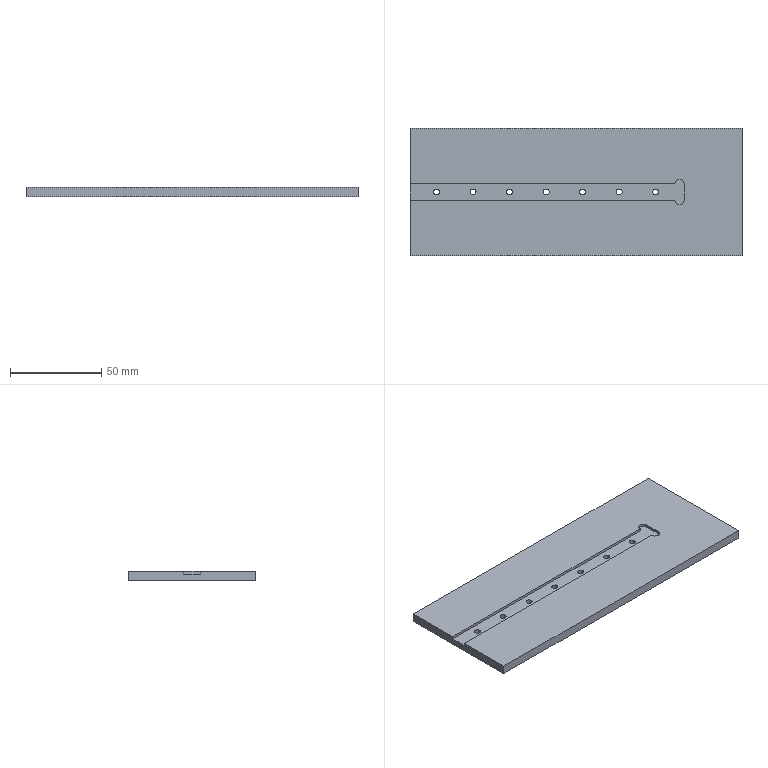Part | STEP file | Handling mechanism support plate | 1 solid | 26 faces | box 181.74 x 70 x 5 mm | volume 61345 mm3 | cylinder 16 | plane 10 | commonest cylinder face diameters 3.3 x14 5 x2
STEP:
#1=CARTESIAN_POINT('',(45.28,0.,0.));
#2=VERTEX_POINT('',#1);
#3=CARTESIAN_POINT('',(41.98,0.,0.));
#4=VERTEX_POINT('',#3);
#5=CARTESIAN_POINT('',(43.63,0.,0.));
#6=DIRECTION('',(0.,0.,-1.));
#7=DIRECTION('',(-1.,0.,0.));
#8=AXIS2_PLACEMENT_3D('',#5,#6,#7);
#9=CIRCLE('',#8,1.65);
#10=EDGE_CURVE('',#2,#4,#9,.T.);
#11=ORIENTED_EDGE('',*,*,#10,.T.);
#12=CARTESIAN_POINT('',(41.98,0.,3.5));
#13=VERTEX_POINT('',#12);
#14=CARTESIAN_POINT('',(41.98,0.,5.));
#15=DIRECTION('',(0.,0.,1.));
#16=VECTOR('',#15,1000.);
#17=LINE('',#14,#16);
#18=EDGE_CURVE('',#4,#13,#17,.T.);
#19=ORIENTED_EDGE('',*,*,#18,.T.);
#20=CARTESIAN_POINT('',(45.28,0.,3.5));
#21=VERTEX_POINT('',#20);
#22=CARTESIAN_POINT('',(43.63,0.,3.5));
#23=DIRECTION('',(0.,0.,1.));
#24=DIRECTION('',(1.,0.,0.));
#25=AXIS2_PLACEMENT_3D('',#22,#23,#24);
#26=CIRCLE('',#25,1.65);
#27=EDGE_CURVE('',#13,#21,#26,.T.);
#28=ORIENTED_EDGE('',*,*,#27,.T.);
#29=CARTESIAN_POINT('',(45.28,0.,5.));
#30=DIRECTION('',(0.,0.,1.));
#31=VECTOR('',#30,1000.);
#32=LINE('',#29,#31);
#33=EDGE_CURVE('',#2,#21,#32,.T.);
#34=ORIENTED_EDGE('',*,*,#33,.F.);
#35=EDGE_LOOP('',(#11,#19,#28,#34));
#36=FACE_OUTER_BOUND('',#35,.T.);
#37=CARTESIAN_POINT('',(43.63,0.,5.));
#38=DIRECTION('',(0.,0.,1.));
#39=DIRECTION('',(1.,0.,0.));
#40=AXIS2_PLACEMENT_3D('',#37,#38,#39);
#41=CYLINDRICAL_SURFACE('',#40,1.65);
#42=ADVANCED_FACE('',(#36),#41,.F.);
#43=CARTESIAN_POINT('',(25.28,0.,0.));
#44=VERTEX_POINT('',#43);
#45=CARTESIAN_POINT('',(21.98,0.,0.));
#46=VERTEX_POINT('',#45);
#47=CARTESIAN_POINT('',(23.63,0.,0.));
#48=DIRECTION('',(0.,0.,-1.));
#49=DIRECTION('',(-1.,0.,0.));
#50=AXIS2_PLACEMENT_3D('',#47,#48,#49);
#51=CIRCLE('',#50,1.65);
#52=EDGE_CURVE('',#44,#46,#51,.T.);
#53=ORIENTED_EDGE('',*,*,#52,.T.);
#54=CARTESIAN_POINT('',(21.98,0.,3.5));
#55=VERTEX_POINT('',#54);
#56=CARTESIAN_POINT('',(21.98,0.,5.));
#57=DIRECTION('',(0.,0.,1.));
#58=VECTOR('',#57,1000.);
#59=LINE('',#56,#58);
#60=EDGE_CURVE('',#46,#55,#59,.T.);
#61=ORIENTED_EDGE('',*,*,#60,.T.);
#62=CARTESIAN_POINT('',(25.28,0.,3.5));
#63=VERTEX_POINT('',#62);
#64=CARTESIAN_POINT('',(23.63,0.,3.5));
#65=DIRECTION('',(0.,0.,1.));
#66=DIRECTION('',(1.,0.,0.));
#67=AXIS2_PLACEMENT_3D('',#64,#65,#66);
#68=CIRCLE('',#67,1.65);
#69=EDGE_CURVE('',#55,#63,#68,.T.);
#70=ORIENTED_EDGE('',*,*,#69,.T.);
#71=CARTESIAN_POINT('',(25.28,0.,5.));
#72=DIRECTION('',(0.,0.,1.));
#73=VECTOR('',#72,1000.);
#74=LINE('',#71,#73);
#75=EDGE_CURVE('',#44,#63,#74,.T.);
#76=ORIENTED_EDGE('',*,*,#75,.F.);
#77=EDGE_LOOP('',(#53,#61,#70,#76));
#78=FACE_OUTER_BOUND('',#77,.T.);
#79=CARTESIAN_POINT('',(23.63,0.,5.));
#80=DIRECTION('',(0.,0.,1.));
#81=DIRECTION('',(1.,0.,0.));
#82=AXIS2_PLACEMENT_3D('',#79,#80,#81);
#83=CYLINDRICAL_SURFACE('',#82,1.65);
#84=ADVANCED_FACE('',(#78),#83,.F.);
#85=CARTESIAN_POINT('',(5.28,0.,0.));
#86=VERTEX_POINT('',#85);
#87=CARTESIAN_POINT('',(1.98,0.,0.));
#88=VERTEX_POINT('',#87);
#89=CARTESIAN_POINT('',(3.63,0.,0.));
#90=DIRECTION('',(0.,0.,-1.));
#91=DIRECTION('',(-1.,0.,0.));
#92=AXIS2_PLACEMENT_3D('',#89,#90,#91);
#93=CIRCLE('',#92,1.65);
#94=EDGE_CURVE('',#86,#88,#93,.T.);
#95=ORIENTED_EDGE('',*,*,#94,.T.);
#96=CARTESIAN_POINT('',(1.98,0.,3.5));
#97=VERTEX_POINT('',#96);
#98=CARTESIAN_POINT('',(1.98,0.,5.));
#99=DIRECTION('',(0.,0.,1.));
#100=VECTOR('',#99,1000.);
#101=LINE('',#98,#100);
#102=EDGE_CURVE('',#88,#97,#101,.T.);
#103=ORIENTED_EDGE('',*,*,#102,.T.);
#104=CARTESIAN_POINT('',(5.28,0.,3.5));
#105=VERTEX_POINT('',#104);
#106=CARTESIAN_POINT('',(3.63,0.,3.5));
#107=DIRECTION('',(0.,0.,1.));
#108=DIRECTION('',(1.,0.,0.));
#109=AXIS2_PLACEMENT_3D('',#106,#107,#108);
#110=CIRCLE('',#109,1.65);
#111=EDGE_CURVE('',#97,#105,#110,.T.);
#112=ORIENTED_EDGE('',*,*,#111,.T.);
#113=CARTESIAN_POINT('',(5.28,0.,5.));
#114=DIRECTION('',(0.,0.,1.));
#115=VECTOR('',#114,1000.);
#116=LINE('',#113,#115);
#117=EDGE_CURVE('',#86,#105,#116,.T.);
#118=ORIENTED_EDGE('',*,*,#117,.F.);
#119=EDGE_LOOP('',(#95,#103,#112,#118));
#120=FACE_OUTER_BOUND('',#119,.T.);
#121=CARTESIAN_POINT('',(3.63,0.,5.));
#122=DIRECTION('',(0.,0.,1.));
#123=DIRECTION('',(1.,0.,0.));
#124=AXIS2_PLACEMENT_3D('',#121,#122,#123);
#125=CYLINDRICAL_SURFACE('',#124,1.65);
#126=ADVANCED_FACE('',(#120),#125,.F.);
#127=CARTESIAN_POINT('',(-14.72,0.,0.));
#128=VERTEX_POINT('',#127);
#129=CARTESIAN_POINT('',(-18.02,0.,0.));
#130=VERTEX_POINT('',#129);
#131=CARTESIAN_POINT('',(-16.37,0.,0.));
#132=DIRECTION('',(0.,0.,-1.));
#133=DIRECTION('',(-1.,0.,0.));
#134=AXIS2_PLACEMENT_3D('',#131,#132,#133);
#135=CIRCLE('',#134,1.65);
#136=EDGE_CURVE('',#128,#130,#135,.T.);
#137=ORIENTED_EDGE('',*,*,#136,.T.);
#138=CARTESIAN_POINT('',(-18.02,0.,3.5));
#139=VERTEX_POINT('',#138);
#140=CARTESIAN_POINT('',(-18.02,0.,5.));
#141=DIRECTION('',(0.,0.,1.));
#142=VECTOR('',#141,1000.);
#143=LINE('',#140,#142);
#144=EDGE_CURVE('',#130,#139,#143,.T.);
#145=ORIENTED_EDGE('',*,*,#144,.T.);
#146=CARTESIAN_POINT('',(-14.72,0.,3.5));
#147=VERTEX_POINT('',#146);
#148=CARTESIAN_POINT('',(-16.37,0.,3.5));
#149=DIRECTION('',(0.,0.,1.));
#150=DIRECTION('',(1.,0.,0.));
#151=AXIS2_PLACEMENT_3D('',#148,#149,#150);
#152=CIRCLE('',#151,1.65);
#153=EDGE_CURVE('',#139,#147,#152,.T.);
#154=ORIENTED_EDGE('',*,*,#153,.T.);
#155=CARTESIAN_POINT('',(-14.72,0.,5.));
#156=DIRECTION('',(0.,0.,1.));
#157=VECTOR('',#156,1000.);
#158=LINE('',#155,#157);
#159=EDGE_CURVE('',#128,#147,#158,.T.);
#160=ORIENTED_EDGE('',*,*,#159,.F.);
#161=EDGE_LOOP('',(#137,#145,#154,#160));
#162=FACE_OUTER_BOUND('',#161,.T.);
#163=CARTESIAN_POINT('',(-16.37,0.,5.));
#164=DIRECTION('',(0.,0.,1.));
#165=DIRECTION('',(1.,0.,0.));
#166=AXIS2_PLACEMENT_3D('',#163,#164,#165);
#167=CYLINDRICAL_SURFACE('',#166,1.65);
#168=ADVANCED_FACE('',(#162),#167,.F.);
#169=CARTESIAN_POINT('',(-34.72,0.,0.));
#170=VERTEX_POINT('',#169);
#171=CARTESIAN_POINT('',(-38.02,0.,0.));
#172=VERTEX_POINT('',#171);
#173=CARTESIAN_POINT('',(-36.37,0.,0.));
#174=DIRECTION('',(0.,0.,-1.));
#175=DIRECTION('',(-1.,0.,0.));
#176=AXIS2_PLACEMENT_3D('',#173,#174,#175);
#177=CIRCLE('',#176,1.65);
#178=EDGE_CURVE('',#170,#172,#177,.T.);
#179=ORIENTED_EDGE('',*,*,#178,.T.);
#180=CARTESIAN_POINT('',(-38.02,0.,3.5));
#181=VERTEX_POINT('',#180);
#182=CARTESIAN_POINT('',(-38.02,0.,5.));
#183=DIRECTION('',(0.,0.,1.));
#184=VECTOR('',#183,1000.);
#185=LINE('',#182,#184);
#186=EDGE_CURVE('',#172,#181,#185,.T.);
#187=ORIENTED_EDGE('',*,*,#186,.T.);
#188=CARTESIAN_POINT('',(-34.72,0.,3.5));
#189=VERTEX_POINT('',#188);
#190=CARTESIAN_POINT('',(-36.37,0.,3.5));
#191=DIRECTION('',(0.,0.,1.));
#192=DIRECTION('',(1.,0.,0.));
#193=AXIS2_PLACEMENT_3D('',#190,#191,#192);
#194=CIRCLE('',#193,1.65);
#195=EDGE_CURVE('',#181,#189,#194,.T.);
#196=ORIENTED_EDGE('',*,*,#195,.T.);
#197=CARTESIAN_POINT('',(-34.72,0.,5.));
#198=DIRECTION('',(0.,0.,1.));
#199=VECTOR('',#198,1000.);
#200=LINE('',#197,#199);
#201=EDGE_CURVE('',#170,#189,#200,.T.);
#202=ORIENTED_EDGE('',*,*,#201,.F.);
#203=EDGE_LOOP('',(#179,#187,#196,#202));
#204=FACE_OUTER_BOUND('',#203,.T.);
#205=CARTESIAN_POINT('',(-36.37,0.,5.));
#206=DIRECTION('',(0.,0.,1.));
#207=DIRECTION('',(1.,0.,0.));
#208=AXIS2_PLACEMENT_3D('',#205,#206,#207);
#209=CYLINDRICAL_SURFACE('',#208,1.65);
#210=ADVANCED_FACE('',(#204),#209,.F.);
#211=CARTESIAN_POINT('',(-54.72,0.,0.));
#212=VERTEX_POINT('',#211);
#213=CARTESIAN_POINT('',(-58.02,0.,0.));
#214=VERTEX_POINT('',#213);
#215=CARTESIAN_POINT('',(-56.37,0.,0.));
#216=DIRECTION('',(0.,0.,-1.));
#217=DIRECTION('',(-1.,0.,0.));
#218=AXIS2_PLACEMENT_3D('',#215,#216,#217);
#219=CIRCLE('',#218,1.65);
#220=EDGE_CURVE('',#212,#214,#219,.T.);
#221=ORIENTED_EDGE('',*,*,#220,.T.);
#222=CARTESIAN_POINT('',(-58.02,0.,3.5));
#223=VERTEX_POINT('',#222);
#224=CARTESIAN_POINT('',(-58.02,0.,5.));
#225=DIRECTION('',(0.,0.,1.));
#226=VECTOR('',#225,1000.);
#227=LINE('',#224,#226);
#228=EDGE_CURVE('',#214,#223,#227,.T.);
#229=ORIENTED_EDGE('',*,*,#228,.T.);
#230=CARTESIAN_POINT('',(-54.72,0.,3.5));
#231=VERTEX_POINT('',#230);
#232=CARTESIAN_POINT('',(-56.37,0.,3.5));
#233=DIRECTION('',(0.,0.,1.));
#234=DIRECTION('',(1.,0.,0.));
#235=AXIS2_PLACEMENT_3D('',#232,#233,#234);
#236=CIRCLE('',#235,1.65);
#237=EDGE_CURVE('',#223,#231,#236,.T.);
#238=ORIENTED_EDGE('',*,*,#237,.T.);
#239=CARTESIAN_POINT('',(-54.72,0.,5.));
#240=DIRECTION('',(0.,0.,1.));
#241=VECTOR('',#240,1000.);
#242=LINE('',#239,#241);
#243=EDGE_CURVE('',#212,#231,#242,.T.);
#244=ORIENTED_EDGE('',*,*,#243,.F.);
#245=EDGE_LOOP('',(#221,#229,#238,#244));
#246=FACE_OUTER_BOUND('',#245,.T.);
#247=CARTESIAN_POINT('',(-56.37,0.,5.));
#248=DIRECTION('',(0.,0.,1.));
#249=DIRECTION('',(1.,0.,0.));
#250=AXIS2_PLACEMENT_3D('',#247,#248,#249);
#251=CYLINDRICAL_SURFACE('',#250,1.65);
#252=ADVANCED_FACE('',(#246),#251,.F.);
#253=CARTESIAN_POINT('',(-74.72,0.,0.));
#254=VERTEX_POINT('',#253);
#255=CARTESIAN_POINT('',(-78.02,0.,0.));
#256=VERTEX_POINT('',#255);
#257=CARTESIAN_POINT('',(-76.37,0.,0.));
#258=DIRECTION('',(0.,0.,-1.));
#259=DIRECTION('',(-1.,0.,0.));
#260=AXIS2_PLACEMENT_3D('',#257,#258,#259);
#261=CIRCLE('',#260,1.65);
#262=EDGE_CURVE('',#254,#256,#261,.T.);
#263=ORIENTED_EDGE('',*,*,#262,.T.);
#264=CARTESIAN_POINT('',(-78.02,0.,3.5));
#265=VERTEX_POINT('',#264);
#266=CARTESIAN_POINT('',(-78.02,0.,5.));
#267=DIRECTION('',(0.,0.,1.));
#268=VECTOR('',#267,1000.);
#269=LINE('',#266,#268);
#270=EDGE_CURVE('',#256,#265,#269,.T.);
#271=ORIENTED_EDGE('',*,*,#270,.T.);
#272=CARTESIAN_POINT('',(-74.72,0.,3.5));
#273=VERTEX_POINT('',#272);
#274=CARTESIAN_POINT('',(-76.37,0.,3.5));
#275=DIRECTION('',(0.,0.,1.));
#276=DIRECTION('',(1.,0.,0.));
#277=AXIS2_PLACEMENT_3D('',#274,#275,#276);
#278=CIRCLE('',#277,1.65);
#279=EDGE_CURVE('',#265,#273,#278,.T.);
#280=ORIENTED_EDGE('',*,*,#279,.T.);
#281=CARTESIAN_POINT('',(-74.72,0.,5.));
#282=DIRECTION('',(0.,0.,1.));
#283=VECTOR('',#282,1000.);
#284=LINE('',#281,#283);
#285=EDGE_CURVE('',#254,#273,#284,.T.);
#286=ORIENTED_EDGE('',*,*,#285,.F.);
#287=EDGE_LOOP('',(#263,#271,#280,#286));
#288=FACE_OUTER_BOUND('',#287,.T.);
#289=CARTESIAN_POINT('',(-76.37,0.,5.));
#290=DIRECTION('',(0.,0.,1.));
#291=DIRECTION('',(1.,0.,0.));
#292=AXIS2_PLACEMENT_3D('',#289,#290,#291);
#293=CYLINDRICAL_SURFACE('',#292,1.65);
#294=ADVANCED_FACE('',(#288),#293,.F.);
#295=CARTESIAN_POINT('',(-90.87,-4.5,5.));
#296=VERTEX_POINT('',#295);
#297=CARTESIAN_POINT('',(-90.87,-35.,5.));
#298=VERTEX_POINT('',#297);
#299=CARTESIAN_POINT('',(-90.87,35.,5.));
#300=DIRECTION('',(0.,-1.,0.));
#301=VECTOR('',#300,1000.);
#302=LINE('',#299,#301);
#303=EDGE_CURVE('',#296,#298,#302,.T.);
#304=ORIENTED_EDGE('',*,*,#303,.F.);
#305=CARTESIAN_POINT('',(-90.87,-4.5,3.5));
#306=VERTEX_POINT('',#305);
#307=CARTESIAN_POINT('',(-90.87,-4.5,3.5));
#308=DIRECTION('',(0.,0.,1.));
#309=VECTOR('',#308,1000.);
#310=LINE('',#307,#309);
#311=EDGE_CURVE('',#306,#296,#310,.T.);
#312=ORIENTED_EDGE('',*,*,#311,.F.);
#313=CARTESIAN_POINT('',(-90.87,4.5,3.5));
#314=VERTEX_POINT('',#313);
#315=CARTESIAN_POINT('',(-90.87,0.,3.5));
#316=DIRECTION('',(0.,-1.,0.));
#317=VECTOR('',#316,1000.);
#318=LINE('',#315,#317);
#319=EDGE_CURVE('',#314,#306,#318,.T.);
#320=ORIENTED_EDGE('',*,*,#319,.F.);
#321=CARTESIAN_POINT('',(-90.87,4.5,5.));
#322=VERTEX_POINT('',#321);
#323=CARTESIAN_POINT('',(-90.87,4.5,3.5));
#324=DIRECTION('',(0.,0.,1.));
#325=VECTOR('',#324,1000.);
#326=LINE('',#323,#325);
#327=EDGE_CURVE('',#314,#322,#326,.T.);
#328=ORIENTED_EDGE('',*,*,#327,.T.);
#329=CARTESIAN_POINT('',(-90.87,35.,5.));
#330=VERTEX_POINT('',#329);
#331=CARTESIAN_POINT('',(-90.87,35.,5.));
#332=DIRECTION('',(0.,-1.,0.));
#333=VECTOR('',#332,1000.);
#334=LINE('',#331,#333);
#335=EDGE_CURVE('',#330,#322,#334,.T.);
#336=ORIENTED_EDGE('',*,*,#335,.F.);
#337=CARTESIAN_POINT('',(-90.87,35.,0.));
#338=VERTEX_POINT('',#337);
#339=CARTESIAN_POINT('',(-90.87,35.,5.));
#340=DIRECTION('',(0.,0.,-1.));
#341=VECTOR('',#340,1000.);
#342=LINE('',#339,#341);
#343=EDGE_CURVE('',#330,#338,#342,.T.);
#344=ORIENTED_EDGE('',*,*,#343,.T.);
#345=CARTESIAN_POINT('',(-90.87,-35.,0.));
#346=VERTEX_POINT('',#345);
#347=CARTESIAN_POINT('',(-90.87,35.,0.));
#348=DIRECTION('',(0.,-1.,0.));
#349=VECTOR('',#348,1000.);
#350=LINE('',#347,#349);
#351=EDGE_CURVE('',#338,#346,#350,.T.);
#352=ORIENTED_EDGE('',*,*,#351,.T.);
#353=CARTESIAN_POINT('',(-90.87,-35.,5.));
#354=DIRECTION('',(0.,0.,-1.));
#355=VECTOR('',#354,1000.);
#356=LINE('',#353,#355);
#357=EDGE_CURVE('',#298,#346,#356,.T.);
#358=ORIENTED_EDGE('',*,*,#357,.F.);
#359=EDGE_LOOP('',(#304,#312,#320,#328,#336,#344,#352,#358));
#360=FACE_OUTER_BOUND('',#359,.T.);
#361=CARTESIAN_POINT('',(-90.87,35.,5.));
#362=DIRECTION('',(1.,0.,0.));
#363=DIRECTION('',(0.,0.,-1.));
#364=AXIS2_PLACEMENT_3D('',#361,#362,#363);
#365=PLANE('',#364);
#366=ADVANCED_FACE('',(#360),#365,.F.);
#367=CARTESIAN_POINT('',(90.87,-35.,0.));
#368=VERTEX_POINT('',#367);
#369=CARTESIAN_POINT('',(90.87,-35.,0.));
#370=DIRECTION('',(1.,0.,0.));
#371=VECTOR('',#370,1000.);
#372=LINE('',#369,#371);
#373=EDGE_CURVE('',#346,#368,#372,.T.);
#374=ORIENTED_EDGE('',*,*,#373,.T.);
#375=CARTESIAN_POINT('',(90.87,-35.,5.));
#376=VERTEX_POINT('',#375);
#377=CARTESIAN_POINT('',(90.87,-35.,5.));
#378=DIRECTION('',(0.,0.,-1.));
#379=VECTOR('',#378,1000.);
#380=LINE('',#377,#379);
#381=EDGE_CURVE('',#376,#368,#380,.T.);
#382=ORIENTED_EDGE('',*,*,#381,.F.);
#383=CARTESIAN_POINT('',(90.87,-35.,5.));
#384=DIRECTION('',(1.,0.,0.));
#385=VECTOR('',#384,1000.);
#386=LINE('',#383,#385);
#387=EDGE_CURVE('',#298,#376,#386,.T.);
#388=ORIENTED_EDGE('',*,*,#387,.F.);
#389=ORIENTED_EDGE('',*,*,#357,.T.);
#390=EDGE_LOOP('',(#374,#382,#388,#389));
#391=FACE_OUTER_BOUND('',#390,.T.);
#392=CARTESIAN_POINT('',(90.87,-35.,5.));
#393=DIRECTION('',(0.,1.,0.));
#394=DIRECTION('',(-1.,0.,0.));
#395=AXIS2_PLACEMENT_3D('',#392,#393,#394);
#396=PLANE('',#395);
#397=ADVANCED_FACE('',(#391),#396,.F.);
#398=CARTESIAN_POINT('',(90.87,35.,0.));
#399=VERTEX_POINT('',#398);
#400=CARTESIAN_POINT('',(90.87,35.,0.));
#401=DIRECTION('',(0.,1.,0.));
#402=VECTOR('',#401,1000.);
#403=LINE('',#400,#402);
#404=EDGE_CURVE('',#368,#399,#403,.T.);
#405=ORIENTED_EDGE('',*,*,#404,.T.);
#406=CARTESIAN_POINT('',(90.87,35.,5.));
#407=VERTEX_POINT('',#406);
#408=CARTESIAN_POINT('',(90.87,35.,5.));
#409=DIRECTION('',(0.,0.,-1.));
#410=VECTOR('',#409,1000.);
#411=LINE('',#408,#410);
#412=EDGE_CURVE('',#407,#399,#411,.T.);
#413=ORIENTED_EDGE('',*,*,#412,.F.);
#414=CARTESIAN_POINT('',(90.87,35.,5.));
#415=DIRECTION('',(0.,1.,0.));
#416=VECTOR('',#415,1000.);
#417=LINE('',#414,#416);
#418=EDGE_CURVE('',#376,#407,#417,.T.);
#419=ORIENTED_EDGE('',*,*,#418,.F.);
#420=ORIENTED_EDGE('',*,*,#381,.T.);
#421=EDGE_LOOP('',(#405,#413,#419,#420));
#422=FACE_OUTER_BOUND('',#421,.T.);
#423=CARTESIAN_POINT('',(90.87,35.,5.));
#424=DIRECTION('',(-1.,0.,0.));
#425=DIRECTION('',(0.,0.,1.));
#426=AXIS2_PLACEMENT_3D('',#423,#424,#425);
#427=PLANE('',#426);
#428=ADVANCED_FACE('',(#422),#427,.F.);
#429=CARTESIAN_POINT('',(90.87,35.,0.));
#430=DIRECTION('',(-1.,0.,0.));
#431=VECTOR('',#430,1000.);
#432=LINE('',#429,#431);
#433=EDGE_CURVE('',#399,#338,#432,.T.);
#434=ORIENTED_EDGE('',*,*,#433,.T.);
#435=ORIENTED_EDGE('',*,*,#343,.F.);
#436=CARTESIAN_POINT('',(90.87,35.,5.));
#437=DIRECTION('',(-1.,0.,0.));
#438=VECTOR('',#437,1000.);
#439=LINE('',#436,#438);
#440=EDGE_CURVE('',#407,#330,#439,.T.);
#441=ORIENTED_EDGE('',*,*,#440,.F.);
#442=ORIENTED_EDGE('',*,*,#412,.T.);
#443=EDGE_LOOP('',(#434,#435,#441,#442));
#444=FACE_OUTER_BOUND('',#443,.T.);
#445=CARTESIAN_POINT('',(90.87,35.,5.));
#446=DIRECTION('',(0.,-1.,0.));
#447=DIRECTION('',(1.,0.,0.));
#448=AXIS2_PLACEMENT_3D('',#445,#446,#447);
#449=PLANE('',#448);
#450=ADVANCED_FACE('',(#444),#449,.F.);
#451=CARTESIAN_POINT('',(54.13,-4.5,5.));
#452=VERTEX_POINT('',#451);
#453=CARTESIAN_POINT('',(59.13,-4.5,5.));
#454=VERTEX_POINT('',#453);
#455=CARTESIAN_POINT('',(56.63,-4.5,5.));
#456=DIRECTION('',(0.,0.,1.));
#457=DIRECTION('',(1.,0.,0.));
#458=AXIS2_PLACEMENT_3D('',#455,#456,#457);
#459=CIRCLE('',#458,2.5);
#460=EDGE_CURVE('',#452,#454,#459,.T.);
#461=ORIENTED_EDGE('',*,*,#460,.F.);
#462=CARTESIAN_POINT('',(0.,-4.5,5.));
#463=DIRECTION('',(1.,0.,0.));
#464=VECTOR('',#463,1000.);
#465=LINE('',#462,#464);
#466=EDGE_CURVE('',#296,#452,#465,.T.);
#467=ORIENTED_EDGE('',*,*,#466,.F.);
#468=ORIENTED_EDGE('',*,*,#303,.T.);
#469=ORIENTED_EDGE('',*,*,#387,.T.);
#470=ORIENTED_EDGE('',*,*,#418,.T.);
#471=ORIENTED_EDGE('',*,*,#440,.T.);
#472=ORIENTED_EDGE('',*,*,#335,.T.);
#473=CARTESIAN_POINT('',(54.13,4.5,5.));
#474=VERTEX_POINT('',#473);
#475=CARTESIAN_POINT('',(0.,4.5,5.));
#476=DIRECTION('',(1.,0.,0.));
#477=VECTOR('',#476,1000.);
#478=LINE('',#475,#477);
#479=EDGE_CURVE('',#322,#474,#478,.T.);
#480=ORIENTED_EDGE('',*,*,#479,.T.);
#481=CARTESIAN_POINT('',(59.13,4.5,5.));
#482=VERTEX_POINT('',#481);
#483=CARTESIAN_POINT('',(56.63,4.5,5.));
#484=DIRECTION('',(0.,0.,1.));
#485=DIRECTION('',(1.,0.,0.));
#486=AXIS2_PLACEMENT_3D('',#483,#484,#485);
#487=CIRCLE('',#486,2.5);
#488=EDGE_CURVE('',#482,#474,#487,.T.);
#489=ORIENTED_EDGE('',*,*,#488,.F.);
#490=CARTESIAN_POINT('',(59.13,0.,5.));
#491=DIRECTION('',(0.,-1.,0.));
#492=VECTOR('',#491,1000.);
#493=LINE('',#490,#492);
#494=EDGE_CURVE('',#482,#454,#493,.T.);
#495=ORIENTED_EDGE('',*,*,#494,.T.);
#496=EDGE_LOOP('',(#461,#467,#468,#469,#470,#471,#472,#480,#489,#495));
#497=FACE_OUTER_BOUND('',#496,.T.);
#498=CARTESIAN_POINT('',(0.,0.,5.));
#499=DIRECTION('',(0.,0.,-1.));
#500=DIRECTION('',(-1.,0.,0.));
#501=AXIS2_PLACEMENT_3D('',#498,#499,#500);
#502=PLANE('',#501);
#503=ADVANCED_FACE('',(#497),#502,.F.);
#504=ORIENTED_EDGE('',*,*,#10,.F.);
#505=CARTESIAN_POINT('',(43.63,0.,0.));
#506=DIRECTION('',(0.,0.,-1.));
#507=DIRECTION('',(-1.,0.,0.));
#508=AXIS2_PLACEMENT_3D('',#505,#506,#507);
#509=CIRCLE('',#508,1.65);
#510=EDGE_CURVE('',#4,#2,#509,.T.);
#511=ORIENTED_EDGE('',*,*,#510,.F.);
#512=EDGE_LOOP('',(#504,#511));
#513=FACE_BOUND('',#512,.T.);
#514=ORIENTED_EDGE('',*,*,#52,.F.);
#515=CARTESIAN_POINT('',(23.63,0.,0.));
#516=DIRECTION('',(0.,0.,-1.));
#517=DIRECTION('',(-1.,0.,0.));
#518=AXIS2_PLACEMENT_3D('',#515,#516,#517);
#519=CIRCLE('',#518,1.65);
#520=EDGE_CURVE('',#46,#44,#519,.T.);
#521=ORIENTED_EDGE('',*,*,#520,.F.);
#522=EDGE_LOOP('',(#514,#521));
#523=FACE_BOUND('',#522,.T.);
#524=ORIENTED_EDGE('',*,*,#94,.F.);
#525=CARTESIAN_POINT('',(3.63,0.,0.));
#526=DIRECTION('',(0.,0.,-1.));
#527=DIRECTION('',(-1.,0.,0.));
#528=AXIS2_PLACEMENT_3D('',#525,#526,#527);
#529=CIRCLE('',#528,1.65);
#530=EDGE_CURVE('',#88,#86,#529,.T.);
#531=ORIENTED_EDGE('',*,*,#530,.F.);
#532=EDGE_LOOP('',(#524,#531));
#533=FACE_BOUND('',#532,.T.);
#534=ORIENTED_EDGE('',*,*,#136,.F.);
#535=CARTESIAN_POINT('',(-16.37,0.,0.));
#536=DIRECTION('',(0.,0.,-1.));
#537=DIRECTION('',(-1.,0.,0.));
#538=AXIS2_PLACEMENT_3D('',#535,#536,#537);
#539=CIRCLE('',#538,1.65);
#540=EDGE_CURVE('',#130,#128,#539,.T.);
#541=ORIENTED_EDGE('',*,*,#540,.F.);
#542=EDGE_LOOP('',(#534,#541));
#543=FACE_BOUND('',#542,.T.);
#544=ORIENTED_EDGE('',*,*,#178,.F.);
#545=CARTESIAN_POINT('',(-36.37,0.,0.));
#546=DIRECTION('',(0.,0.,-1.));
#547=DIRECTION('',(-1.,0.,0.));
#548=AXIS2_PLACEMENT_3D('',#545,#546,#547);
#549=CIRCLE('',#548,1.65);
#550=EDGE_CURVE('',#172,#170,#549,.T.);
#551=ORIENTED_EDGE('',*,*,#550,.F.);
#552=EDGE_LOOP('',(#544,#551));
#553=FACE_BOUND('',#552,.T.);
#554=ORIENTED_EDGE('',*,*,#220,.F.);
#555=CARTESIAN_POINT('',(-56.37,0.,0.));
#556=DIRECTION('',(0.,0.,-1.));
#557=DIRECTION('',(-1.,0.,0.));
#558=AXIS2_PLACEMENT_3D('',#555,#556,#557);
#559=CIRCLE('',#558,1.65);
#560=EDGE_CURVE('',#214,#212,#559,.T.);
#561=ORIENTED_EDGE('',*,*,#560,.F.);
#562=EDGE_LOOP('',(#554,#561));
#563=FACE_BOUND('',#562,.T.);
#564=ORIENTED_EDGE('',*,*,#262,.F.);
#565=CARTESIAN_POINT('',(-76.37,0.,0.));
#566=DIRECTION('',(0.,0.,-1.));
#567=DIRECTION('',(-1.,0.,0.));
#568=AXIS2_PLACEMENT_3D('',#565,#566,#567);
#569=CIRCLE('',#568,1.65);
#570=EDGE_CURVE('',#256,#254,#569,.T.);
#571=ORIENTED_EDGE('',*,*,#570,.F.);
#572=EDGE_LOOP('',(#564,#571));
#573=FACE_BOUND('',#572,.T.);
#574=ORIENTED_EDGE('',*,*,#351,.F.);
#575=ORIENTED_EDGE('',*,*,#433,.F.);
#576=ORIENTED_EDGE('',*,*,#404,.F.);
#577=ORIENTED_EDGE('',*,*,#373,.F.);
#578=EDGE_LOOP('',(#574,#575,#576,#577));
#579=FACE_OUTER_BOUND('',#578,.T.);
#580=CARTESIAN_POINT('',(0.,0.,0.));
#581=DIRECTION('',(0.,0.,-1.));
#582=DIRECTION('',(-1.,0.,0.));
#583=AXIS2_PLACEMENT_3D('',#580,#581,#582);
#584=PLANE('',#583);
#585=ADVANCED_FACE('',(#513,#523,#533,#543,#553,#563,#573,#579),#584,.T.);
#586=ORIENTED_EDGE('',*,*,#460,.T.);
#587=CARTESIAN_POINT('',(59.13,-4.5,3.5));
#588=VERTEX_POINT('',#587);
#589=CARTESIAN_POINT('',(59.13,-4.5,3.5));
#590=DIRECTION('',(0.,0.,1.));
#591=VECTOR('',#590,1000.);
#592=LINE('',#589,#591);
#593=EDGE_CURVE('',#588,#454,#592,.T.);
#594=ORIENTED_EDGE('',*,*,#593,.F.);
#595=CARTESIAN_POINT('',(54.13,-4.5,3.5));
#596=VERTEX_POINT('',#595);
#597=CARTESIAN_POINT('',(56.63,-4.5,3.5));
#598=DIRECTION('',(0.,0.,1.));
#599=DIRECTION('',(1.,0.,0.));
#600=AXIS2_PLACEMENT_3D('',#597,#598,#599);
#601=CIRCLE('',#600,2.5);
#602=EDGE_CURVE('',#596,#588,#601,.T.);
#603=ORIENTED_EDGE('',*,*,#602,.F.);
#604=CARTESIAN_POINT('',(54.13,-4.5,3.5));
#605=DIRECTION('',(0.,0.,1.));
#606=VECTOR('',#605,1000.);
#607=LINE('',#604,#606);
#608=EDGE_CURVE('',#596,#452,#607,.T.);
#609=ORIENTED_EDGE('',*,*,#608,.T.);
#610=EDGE_LOOP('',(#586,#594,#603,#609));
#611=FACE_OUTER_BOUND('',#610,.T.);
#612=CARTESIAN_POINT('',(56.63,-4.5,3.5));
#613=DIRECTION('',(0.,0.,1.));
#614=DIRECTION('',(1.,0.,0.));
#615=AXIS2_PLACEMENT_3D('',#612,#613,#614);
#616=CYLINDRICAL_SURFACE('',#615,2.5);
#617=ADVANCED_FACE('',(#611),#616,.F.);
#618=ORIENTED_EDGE('',*,*,#466,.T.);
#619=ORIENTED_EDGE('',*,*,#608,.F.);
#620=CARTESIAN_POINT('',(0.,-4.5,3.5));
#621=DIRECTION('',(1.,0.,0.));
#622=VECTOR('',#621,1000.);
#623=LINE('',#620,#622);
#624=EDGE_CURVE('',#306,#596,#623,.T.);
#625=ORIENTED_EDGE('',*,*,#624,.F.);
#626=ORIENTED_EDGE('',*,*,#311,.T.);
#627=EDGE_LOOP('',(#618,#619,#625,#626));
#628=FACE_OUTER_BOUND('',#627,.T.);
#629=CARTESIAN_POINT('',(0.,-4.5,3.5));
#630=DIRECTION('',(0.,-1.,0.));
#631=DIRECTION('',(0.,0.,-1.));
#632=AXIS2_PLACEMENT_3D('',#629,#630,#631);
#633=PLANE('',#632);
#634=ADVANCED_FACE('',(#628),#633,.F.);
#635=ORIENTED_EDGE('',*,*,#479,.F.);
#636=ORIENTED_EDGE('',*,*,#327,.F.);
#637=CARTESIAN_POINT('',(54.13,4.5,3.5));
#638=VERTEX_POINT('',#637);
#639=CARTESIAN_POINT('',(0.,4.5,3.5));
#640=DIRECTION('',(1.,0.,0.));
#641=VECTOR('',#640,1000.);
#642=LINE('',#639,#641);
#643=EDGE_CURVE('',#314,#638,#642,.T.);
#644=ORIENTED_EDGE('',*,*,#643,.T.);
#645=CARTESIAN_POINT('',(54.13,4.5,3.5));
#646=DIRECTION('',(0.,0.,1.));
#647=VECTOR('',#646,1000.);
#648=LINE('',#645,#647);
#649=EDGE_CURVE('',#638,#474,#648,.T.);
#650=ORIENTED_EDGE('',*,*,#649,.T.);
#651=EDGE_LOOP('',(#635,#636,#644,#650));
#652=FACE_OUTER_BOUND('',#651,.T.);
#653=CARTESIAN_POINT('',(0.,4.5,3.5));
#654=DIRECTION('',(0.,-1.,0.));
#655=DIRECTION('',(0.,0.,-1.));
#656=AXIS2_PLACEMENT_3D('',#653,#654,#655);
#657=PLANE('',#656);
#658=ADVANCED_FACE('',(#652),#657,.T.);
#659=ORIENTED_EDGE('',*,*,#488,.T.);
#660=ORIENTED_EDGE('',*,*,#649,.F.);
#661=CARTESIAN_POINT('',(59.13,4.5,3.5));
#662=VERTEX_POINT('',#661);
#663=CARTESIAN_POINT('',(56.63,4.5,3.5));
#664=DIRECTION('',(0.,0.,1.));
#665=DIRECTION('',(1.,0.,0.));
#666=AXIS2_PLACEMENT_3D('',#663,#664,#665);
#667=CIRCLE('',#666,2.5);
#668=EDGE_CURVE('',#662,#638,#667,.T.);
#669=ORIENTED_EDGE('',*,*,#668,.F.);
#670=CARTESIAN_POINT('',(59.13,4.5,3.5));
#671=DIRECTION('',(0.,0.,1.));
#672=VECTOR('',#671,1000.);
#673=LINE('',#670,#672);
#674=EDGE_CURVE('',#662,#482,#673,.T.);
#675=ORIENTED_EDGE('',*,*,#674,.T.);
#676=EDGE_LOOP('',(#659,#660,#669,#675));
#677=FACE_OUTER_BOUND('',#676,.T.);
#678=CARTESIAN_POINT('',(56.63,4.5,3.5));
#679=DIRECTION('',(0.,0.,1.));
#680=DIRECTION('',(1.,0.,0.));
#681=AXIS2_PLACEMENT_3D('',#678,#679,#680);
#682=CYLINDRICAL_SURFACE('',#681,2.5);
#683=ADVANCED_FACE('',(#677),#682,.F.);
#684=ORIENTED_EDGE('',*,*,#494,.F.);
#685=ORIENTED_EDGE('',*,*,#674,.F.);
#686=CARTESIAN_POINT('',(59.13,0.,3.5));
#687=DIRECTION('',(0.,-1.,0.));
#688=VECTOR('',#687,1000.);
#689=LINE('',#686,#688);
#690=EDGE_CURVE('',#662,#588,#689,.T.);
#691=ORIENTED_EDGE('',*,*,#690,.T.);
#692=ORIENTED_EDGE('',*,*,#593,.T.);
#693=EDGE_LOOP('',(#684,#685,#691,#692));
#694=FACE_OUTER_BOUND('',#693,.T.);
#695=CARTESIAN_POINT('',(59.13,0.,3.5));
#696=DIRECTION('',(-1.,0.,0.));
#697=DIRECTION('',(0.,0.,1.));
#698=AXIS2_PLACEMENT_3D('',#695,#696,#697);
#699=PLANE('',#698);
#700=ADVANCED_FACE('',(#694),#699,.T.);
#701=CARTESIAN_POINT('',(43.63,0.,3.5));
#702=DIRECTION('',(0.,0.,1.));
#703=DIRECTION('',(1.,0.,0.));
#704=AXIS2_PLACEMENT_3D('',#701,#702,#703);
#705=CIRCLE('',#704,1.65);
#706=EDGE_CURVE('',#21,#13,#705,.T.);
#707=ORIENTED_EDGE('',*,*,#706,.F.);
#708=ORIENTED_EDGE('',*,*,#27,.F.);
#709=EDGE_LOOP('',(#707,#708));
#710=FACE_BOUND('',#709,.T.);
#711=CARTESIAN_POINT('',(23.63,0.,3.5));
#712=DIRECTION('',(0.,0.,1.));
#713=DIRECTION('',(1.,0.,0.));
#714=AXIS2_PLACEMENT_3D('',#711,#712,#713);
#715=CIRCLE('',#714,1.65);
#716=EDGE_CURVE('',#63,#55,#715,.T.);
#717=ORIENTED_EDGE('',*,*,#716,.F.);
#718=ORIENTED_EDGE('',*,*,#69,.F.);
#719=EDGE_LOOP('',(#717,#718));
#720=FACE_BOUND('',#719,.T.);
#721=CARTESIAN_POINT('',(3.63,0.,3.5));
#722=DIRECTION('',(0.,0.,1.));
#723=DIRECTION('',(1.,0.,0.));
#724=AXIS2_PLACEMENT_3D('',#721,#722,#723);
#725=CIRCLE('',#724,1.65);
#726=EDGE_CURVE('',#105,#97,#725,.T.);
#727=ORIENTED_EDGE('',*,*,#726,.F.);
#728=ORIENTED_EDGE('',*,*,#111,.F.);
#729=EDGE_LOOP('',(#727,#728));
#730=FACE_BOUND('',#729,.T.);
#731=CARTESIAN_POINT('',(-16.37,0.,3.5));
#732=DIRECTION('',(0.,0.,1.));
#733=DIRECTION('',(1.,0.,0.));
#734=AXIS2_PLACEMENT_3D('',#731,#732,#733);
#735=CIRCLE('',#734,1.65);
#736=EDGE_CURVE('',#147,#139,#735,.T.);
#737=ORIENTED_EDGE('',*,*,#736,.F.);
#738=ORIENTED_EDGE('',*,*,#153,.F.);
#739=EDGE_LOOP('',(#737,#738));
#740=FACE_BOUND('',#739,.T.);
#741=CARTESIAN_POINT('',(-36.37,0.,3.5));
#742=DIRECTION('',(0.,0.,1.));
#743=DIRECTION('',(1.,0.,0.));
#744=AXIS2_PLACEMENT_3D('',#741,#742,#743);
#745=CIRCLE('',#744,1.65);
#746=EDGE_CURVE('',#189,#181,#745,.T.);
#747=ORIENTED_EDGE('',*,*,#746,.F.);
#748=ORIENTED_EDGE('',*,*,#195,.F.);
#749=EDGE_LOOP('',(#747,#748));
#750=FACE_BOUND('',#749,.T.);
#751=CARTESIAN_POINT('',(-56.37,0.,3.5));
#752=DIRECTION('',(0.,0.,1.));
#753=DIRECTION('',(1.,0.,0.));
#754=AXIS2_PLACEMENT_3D('',#751,#752,#753);
#755=CIRCLE('',#754,1.65);
#756=EDGE_CURVE('',#231,#223,#755,.T.);
#757=ORIENTED_EDGE('',*,*,#756,.F.);
#758=ORIENTED_EDGE('',*,*,#237,.F.);
#759=EDGE_LOOP('',(#757,#758));
#760=FACE_BOUND('',#759,.T.);
#761=CARTESIAN_POINT('',(-76.37,0.,3.5));
#762=DIRECTION('',(0.,0.,1.));
#763=DIRECTION('',(1.,0.,0.));
#764=AXIS2_PLACEMENT_3D('',#761,#762,#763);
#765=CIRCLE('',#764,1.65);
#766=EDGE_CURVE('',#273,#265,#765,.T.);
#767=ORIENTED_EDGE('',*,*,#766,.F.);
#768=ORIENTED_EDGE('',*,*,#279,.F.);
#769=EDGE_LOOP('',(#767,#768));
#770=FACE_BOUND('',#769,.T.);
#771=ORIENTED_EDGE('',*,*,#602,.T.);
#772=ORIENTED_EDGE('',*,*,#690,.F.);
#773=ORIENTED_EDGE('',*,*,#668,.T.);
#774=ORIENTED_EDGE('',*,*,#643,.F.);
#775=ORIENTED_EDGE('',*,*,#319,.T.);
#776=ORIENTED_EDGE('',*,*,#624,.T.);
#777=EDGE_LOOP('',(#771,#772,#773,#774,#775,#776));
#778=FACE_OUTER_BOUND('',#777,.T.);
#779=CARTESIAN_POINT('',(0.,0.,3.5));
#780=DIRECTION('',(0.,0.,1.));
#781=DIRECTION('',(1.,0.,0.));
#782=AXIS2_PLACEMENT_3D('',#779,#780,#781);
#783=PLANE('',#782);
#784=ADVANCED_FACE('',(#710,#720,#730,#740,#750,#760,#770,#778),#783,.T.);
#785=ORIENTED_EDGE('',*,*,#270,.F.);
#786=ORIENTED_EDGE('',*,*,#570,.T.);
#787=ORIENTED_EDGE('',*,*,#285,.T.);
#788=ORIENTED_EDGE('',*,*,#766,.T.);
#789=EDGE_LOOP('',(#785,#786,#787,#788));
#790=FACE_OUTER_BOUND('',#789,.T.);
#791=CARTESIAN_POINT('',(-76.37,0.,5.));
#792=DIRECTION('',(0.,0.,1.));
#793=DIRECTION('',(1.,0.,0.));
#794=AXIS2_PLACEMENT_3D('',#791,#792,#793);
#795=CYLINDRICAL_SURFACE('',#794,1.65);
#796=ADVANCED_FACE('',(#790),#795,.F.);
#797=ORIENTED_EDGE('',*,*,#228,.F.);
#798=ORIENTED_EDGE('',*,*,#560,.T.);
#799=ORIENTED_EDGE('',*,*,#243,.T.);
#800=ORIENTED_EDGE('',*,*,#756,.T.);
#801=EDGE_LOOP('',(#797,#798,#799,#800));
#802=FACE_OUTER_BOUND('',#801,.T.);
#803=CARTESIAN_POINT('',(-56.37,0.,5.));
#804=DIRECTION('',(0.,0.,1.));
#805=DIRECTION('',(1.,0.,0.));
#806=AXIS2_PLACEMENT_3D('',#803,#804,#805);
#807=CYLINDRICAL_SURFACE('',#806,1.65);
#808=ADVANCED_FACE('',(#802),#807,.F.);
#809=ORIENTED_EDGE('',*,*,#186,.F.);
#810=ORIENTED_EDGE('',*,*,#550,.T.);
#811=ORIENTED_EDGE('',*,*,#201,.T.);
#812=ORIENTED_EDGE('',*,*,#746,.T.);
#813=EDGE_LOOP('',(#809,#810,#811,#812));
#814=FACE_OUTER_BOUND('',#813,.T.);
#815=CARTESIAN_POINT('',(-36.37,0.,5.));
#816=DIRECTION('',(0.,0.,1.));
#817=DIRECTION('',(1.,0.,0.));
#818=AXIS2_PLACEMENT_3D('',#815,#816,#817);
#819=CYLINDRICAL_SURFACE('',#818,1.65);
#820=ADVANCED_FACE('',(#814),#819,.F.);
#821=ORIENTED_EDGE('',*,*,#144,.F.);
#822=ORIENTED_EDGE('',*,*,#540,.T.);
#823=ORIENTED_EDGE('',*,*,#159,.T.);
#824=ORIENTED_EDGE('',*,*,#736,.T.);
#825=EDGE_LOOP('',(#821,#822,#823,#824));
#826=FACE_OUTER_BOUND('',#825,.T.);
#827=CARTESIAN_POINT('',(-16.37,0.,5.));
#828=DIRECTION('',(0.,0.,1.));
#829=DIRECTION('',(1.,0.,0.));
#830=AXIS2_PLACEMENT_3D('',#827,#828,#829);
#831=CYLINDRICAL_SURFACE('',#830,1.65);
#832=ADVANCED_FACE('',(#826),#831,.F.);
#833=ORIENTED_EDGE('',*,*,#102,.F.);
#834=ORIENTED_EDGE('',*,*,#530,.T.);
#835=ORIENTED_EDGE('',*,*,#117,.T.);
#836=ORIENTED_EDGE('',*,*,#726,.T.);
#837=EDGE_LOOP('',(#833,#834,#835,#836));
#838=FACE_OUTER_BOUND('',#837,.T.);
#839=CARTESIAN_POINT('',(3.63,0.,5.));
#840=DIRECTION('',(0.,0.,1.));
#841=DIRECTION('',(1.,0.,0.));
#842=AXIS2_PLACEMENT_3D('',#839,#840,#841);
#843=CYLINDRICAL_SURFACE('',#842,1.65);
#844=ADVANCED_FACE('',(#838),#843,.F.);
#845=ORIENTED_EDGE('',*,*,#60,.F.);
#846=ORIENTED_EDGE('',*,*,#520,.T.);
#847=ORIENTED_EDGE('',*,*,#75,.T.);
#848=ORIENTED_EDGE('',*,*,#716,.T.);
#849=EDGE_LOOP('',(#845,#846,#847,#848));
#850=FACE_OUTER_BOUND('',#849,.T.);
#851=CARTESIAN_POINT('',(23.63,0.,5.));
#852=DIRECTION('',(0.,0.,1.));
#853=DIRECTION('',(1.,0.,0.));
#854=AXIS2_PLACEMENT_3D('',#851,#852,#853);
#855=CYLINDRICAL_SURFACE('',#854,1.65);
#856=ADVANCED_FACE('',(#850),#855,.F.);
#857=ORIENTED_EDGE('',*,*,#18,.F.);
#858=ORIENTED_EDGE('',*,*,#510,.T.);
#859=ORIENTED_EDGE('',*,*,#33,.T.);
#860=ORIENTED_EDGE('',*,*,#706,.T.);
#861=EDGE_LOOP('',(#857,#858,#859,#860));
#862=FACE_OUTER_BOUND('',#861,.T.);
#863=CARTESIAN_POINT('',(43.63,0.,5.));
#864=DIRECTION('',(0.,0.,1.));
#865=DIRECTION('',(1.,0.,0.));
#866=AXIS2_PLACEMENT_3D('',#863,#864,#865);
#867=CYLINDRICAL_SURFACE('',#866,1.65);
#868=ADVANCED_FACE('',(#862),#867,.F.);
#869=CLOSED_SHELL('',(#42,#84,#126,#168,#210,#252,#294,#366,#397,#428,#450,#503,#585,#617,#634,#658,#683,#700,#784,#796,#808,#820,#832,#844,#856,#868));
#870=MANIFOLD_SOLID_BREP('',#869);
#871=CARTESIAN_POINT('',(0.,0.,0.));
#872=DIRECTION('',(0.,0.,1.));
#873=DIRECTION('',(1.,0.,0.));
#874=AXIS2_PLACEMENT_3D('',#871,#872,#873);
#875=(LENGTH_UNIT()NAMED_UNIT(*)SI_UNIT(.MILLI.,.METRE.));
#876=UNCERTAINTY_MEASURE_WITH_UNIT(LENGTH_MEASURE(0.00001),#875,'','');
#877=(NAMED_UNIT(*)PLANE_ANGLE_UNIT()SI_UNIT($,.RADIAN.));
#878=(NAMED_UNIT(*)SI_UNIT($,.STERADIAN.)SOLID_ANGLE_UNIT());
#879=(GEOMETRIC_REPRESENTATION_CONTEXT(3)GLOBAL_UNCERTAINTY_ASSIGNED_CONTEXT((#876))GLOBAL_UNIT_ASSIGNED_CONTEXT((#875,#877,#878))REPRESENTATION_CONTEXT('',''));
#880=ADVANCED_BREP_SHAPE_REPRESENTATION('',(#870,#874),#879);